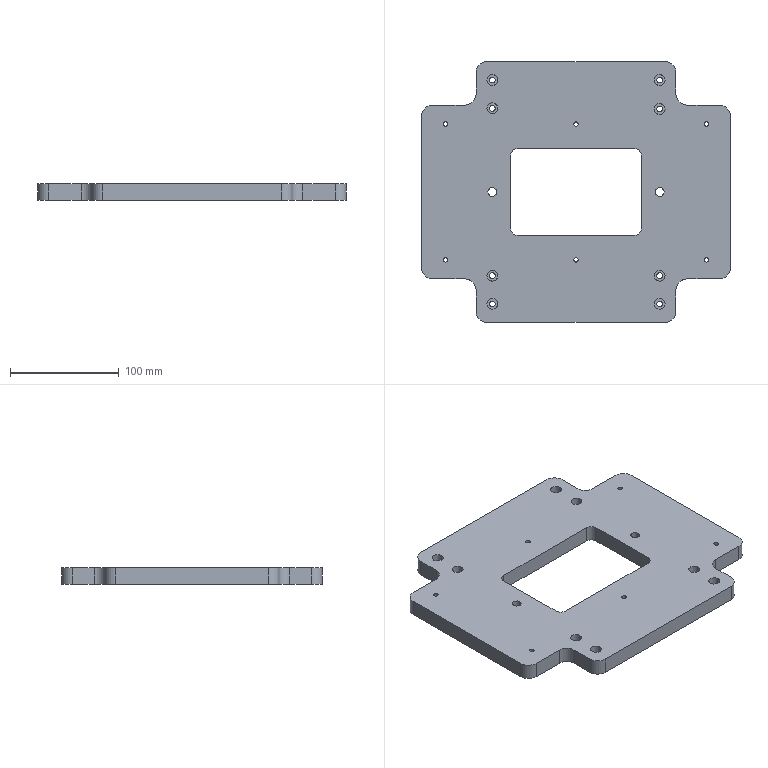NC program | NX | posted with a generic post | part box 284 x 240 x 15 mm
Lines 2693 to 2949 of 2949:
(PLANAR_MILL_1 , TOOL : D6A45)
N5336 T07 M6
N5338 G54
N5340 G17 G0 G90 X-80.743 Y103.766 S9500 M3
N5342 G43 Z30. H7
N5344 Z0.5
N5346 G94 G1 Z-1. F1250.
N5348 G3 X-81.1 Y103. R1.
N5350 X-77. Y98.9 R4.1
N5352 X-81.1 Y103. R-4.1
N5354 X-80.743 Y102.234 R1.
N5356 G1 Z0.5
N5358 G0 Z30.
N5360 Y77.766
N5362 Z0.5
N5364 G1 Z-1.
N5366 G3 X-81.1 Y77. R1.
N5368 X-77. Y72.9 R4.1
N5370 X-81.1 Y77. R-4.1
N5372 X-80.743 Y76.234 R1.
N5374 G1 Z0.5
N5376 G0 Z30.
N5378 X-119.19 Y61.734
N5380 Z0.5
N5382 G1 Z-1.
N5384 G3 X-118.833 Y62.5 R1.
N5386 X-120. Y63.667 R1.167
N5388 X-118.833 Y62.5 R-1.167
N5390 X-119.19 Y63.266 R1.
N5392 G1 Z0.5
N5394 G0 Z30.
N5396 X-74.257 Y-0.766
N5398 Z0.5
N5400 G1 Z-1.
N5402 G3 X-73.9 Y0. R1.
N5404 X-77. Y3.1 R3.1
N5406 X-73.9 Y0. R-3.1
N5408 X-74.257 Y0.766 R1.
N5410 G1 Z0.5
N5412 G0 Z30.
N5414 X-119.19 Y-63.266
N5416 Z0.5
N5418 G1 Z-1.
N5420 G3 X-118.833 Y-62.5 R1.
N5422 X-120. Y-61.333 R1.167
N5424 X-118.833 Y-62.5 R-1.167
N5426 X-119.19 Y-61.734 R1.
N5428 G1 Z0.5
N5430 G0 Z30.
N5432 X-80.743 Y-102.234
N5434 Z0.5
N5436 G1 Z-1.
N5438 G3 X-81.1 Y-103. R1.
N5440 X-77. Y-107.1 R4.1
N5442 X-81.1 Y-103. R-4.1
N5444 X-80.743 Y-103.766 R1.
N5446 G1 Z0.5
N5448 G0 Z30.
N5450 Y-76.234
N5452 Z0.5
N5454 G1 Z-1.
N5456 G3 X-81.1 Y-77. R1.
N5458 X-77. Y-81.1 R4.1
N5460 X-81.1 Y-77. R-4.1
N5462 X-80.743 Y-77.766 R1.
N5464 G1 Z0.5
N5466 G0 Z30.
N5468 X0.81 Y-63.266
N5470 Z0.5
N5472 G1 Z-1.
N5474 G3 X1.167 Y-62.5 R1.
N5476 X0. Y-61.333 R1.167
N5478 X1.167 Y-62.5 R-1.167
N5480 X0.81 Y-61.734 R1.
N5482 G1 Z0.5
N5484 G0 Z30.
N5486 X53.234 Y-38.743
N5488 Z0.5
N5490 G1 Z-1.
N5492 G3 X54. Y-39.1 R1.
N5494 X59.1 Y-34. R5.1
N5496 G1 Y34.
N5498 G3 X54. Y39.1 R5.1
N5500 G1 X-54.
N5502 G3 X-59.1 Y34. R5.1
N5504 G1 Y-34.
N5506 G3 X-54. Y-39.1 R5.1
N5508 G1 X54.
N5510 G3 X54.766 Y-38.743 R1.
N5512 G1 Z0.5
N5514 G0 Z30.
N5516 X-82.766 Y121.257
N5518 Z0.5
N5520 G1 Z-1.
N5522 G3 X-82. Y120.9 R1.
N5524 G1 X82.
N5526 G2 X92.9 Y110. R10.9
N5528 G1 Y90.
N5530 G3 X102. Y80.9 R9.1
N5532 G1 X132.
N5534 G2 X142.9 Y70. R10.9
N5536 G1 Y-70.
N5538 G2 X132. Y-80.9 R10.9
N5540 G1 X102.
N5542 G3 X92.9 Y-90. R9.1
N5544 G1 Y-110.
N5546 G2 X82. Y-120.9 R10.9
N5548 G1 X-82.
N5550 G2 X-92.9 Y-110. R10.9
N5552 G1 Y-90.
N5554 G3 X-102. Y-80.9 R9.1
N5556 G1 X-132.
N5558 G2 X-142.9 Y-70. R10.9
N5560 G1 Y70.
N5562 G2 X-132. Y80.9 R10.9
N5564 G1 X-102.
N5566 G3 X-92.9 Y90. R9.1
N5568 G1 Y110.
N5570 G2 X-82. Y120.9 R10.9
N5572 G3 X-81.234 Y121.257 R1.
N5574 G1 Z0.5
N5576 G0 Z30.
N5578 X0.81 Y61.734
N5580 Z0.5
N5582 G1 Z-1.
N5584 G3 X1.167 Y62.5 R1.
N5586 X0. Y63.667 R1.167
N5588 X1.167 Y62.5 R-1.167
N5590 X0.81 Y63.266 R1.
N5592 G1 Z0.5
N5594 G0 Z30.
N5596 X73.257 Y77.103
N5598 Z0.5
N5600 G1 Z-1.
N5602 G3 X72.9 Y76.337 R1.
N5604 X77. Y72.237 R4.1
N5606 X72.9 Y76.337 R-4.1
N5608 X73.257 Y75.571 R1.
N5610 G1 Z0.5
N5612 G0 Z30.
N5614 Y103.766
N5616 Z0.5
N5618 G1 Z-1.
N5620 G3 X72.9 Y103. R1.
N5622 X77. Y98.9 R4.1
N5624 X72.9 Y103. R-4.1
N5626 X73.257 Y102.234 R1.
N5628 G1 Z0.5
N5630 G0 Z30.
N5632 X120.81 Y61.734
N5634 Z0.5
N5636 G1 Z-1.
N5638 G3 X121.167 Y62.5 R1.
N5640 X120. Y63.667 R1.167
N5642 X121.167 Y62.5 R-1.167
N5644 X120.81 Y63.266 R1.
N5646 G1 Z0.5
N5648 G0 Z30.
N5650 X79.743 Y-0.766
N5652 Z0.5
N5654 G1 Z-1.
N5656 G3 X80.1 Y0. R1.
N5658 X77. Y3.1 R3.1
N5660 X80.1 Y0. R-3.1
N5662 X79.743 Y0.766 R1.
N5664 G1 Z0.5
N5666 G0 Z30.
N5668 X120.81 Y-63.266
N5670 Z0.5
N5672 G1 Z-1.
N5674 G3 X121.167 Y-62.5 R1.
N5676 X120. Y-61.333 R1.167
N5678 X121.167 Y-62.5 R-1.167
N5680 X120.81 Y-61.734 R1.
N5682 G1 Z0.5
N5684 G0 Z30.
N5686 X73.257 Y-76.234
N5688 Z0.5
N5690 G1 Z-1.
N5692 G3 X72.9 Y-77. R1.
N5694 X77. Y-81.1 R4.1
N5696 X72.9 Y-77. R-4.1
N5698 X73.257 Y-77.766 R1.
N5700 G1 Z0.5
N5702 G0 Z30.
N5704 Y-102.234
N5706 Z0.5
N5708 G1 Z-1.
N5710 G3 X72.9 Y-103. R1.
N5712 X77. Y-107.1 R4.1
N5714 X72.9 Y-103. R-4.1
N5716 X73.257 Y-103.766 R1.
N5718 G1 Z0.5
N5720 G0 Z30.
N5722 M5
(刀补6 , TOOL : D6)
N5724 T06 M6
N5726 G54
N5728 G17 G0 G90 X-77. Y0. S9500 M3
N5730 G43 Z30. H6
N5732 Z0.5
N5734 G41 G94 G1 X-76.996 Y-0.1 F1000. D6
N5736 G3 X-76.05 Y0. R0.478
N5738 X-76.05 Y0. Z-0.5 I-0.95 J0.
N5740 X-76.05 Y0. Z-1.5 I-0.95 J0.
N5742 X-76.05 Y0. Z-2.5 I-0.95 J0.
N5744 X-76.05 Y0. Z-3.5 I-0.95 J0.
N5746 X-76.05 Y0. Z-4.5 I-0.95 J0.
N5748 X-76.05 Y0. Z-5.5 I-0.95 J0.
N5750 X-76.05 Y0. Z-6.5 I-0.95 J0.
N5752 X-76.05 Y0. Z-7.5 I-0.95 J0.
N5754 X-76.05 Y0. Z-8.5 I-0.95 J0.
N5756 X-76.05 Y0. Z-9.5 I-0.95 J0.
N5758 X-76.05 Y0. Z-10.5 I-0.95 J0.
N5760 X-76.05 Y0. Z-11.5 I-0.95 J0.
N5762 X-76.05 Y0. Z-12.5 I-0.95 J0.
N5764 X-76.05 Y0. Z-13.5 I-0.95 J0.
N5766 X-76.05 Y0. Z-14.5 I-0.95 J0.
N5768 X-77.95 Y0. Z-15. I-0.95 J0.
N5770 X-77. Y-0.95 R0.95
N5772 X-77.95 Y0. R-0.95
N5774 X-77.004 Y-0.1 R0.478
N5776 G40
N5778 G1 X-77. Y0.
N5780 G0 Z30.
N5782 X77.
N5784 Z0.5
N5786 G41 G1 X77.004 Y-0.1
N5788 G3 X77.95 Y0. R0.478
N5790 X77.95 Y0. Z-0.5 I-0.95 J0.
N5792 X77.95 Y0. Z-1.5 I-0.95 J0.
N5794 X77.95 Y0. Z-2.5 I-0.95 J0.
N5796 X77.95 Y0. Z-3.5 I-0.95 J0.
N5798 X77.95 Y0. Z-4.5 I-0.95 J0.
N5800 X77.95 Y0. Z-5.5 I-0.95 J0.
N5802 X77.95 Y0. Z-6.5 I-0.95 J0.
N5804 X77.95 Y0. Z-7.5 I-0.95 J0.
N5806 X77.95 Y0. Z-8.5 I-0.95 J0.
N5808 X77.95 Y0. Z-9.5 I-0.95 J0.
N5810 X77.95 Y0. Z-10.5 I-0.95 J0.
N5812 X77.95 Y0. Z-11.5 I-0.95 J0.
N5814 X77.95 Y0. Z-12.5 I-0.95 J0.
N5816 X77.95 Y0. Z-13.5 I-0.95 J0.
N5818 X77.95 Y0. Z-14.5 I-0.95 J0.
N5820 X76.05 Y0. Z-15. I-0.95 J0.
N5822 X77. Y-0.95 R0.95
N5824 X76.05 Y0. R-0.95
N5826 X76.996 Y-0.1 R0.478
N5828 G40
N5830 G1 X77. Y0.
N5832 G0 Z30.
N5834 M5
N5836 M2